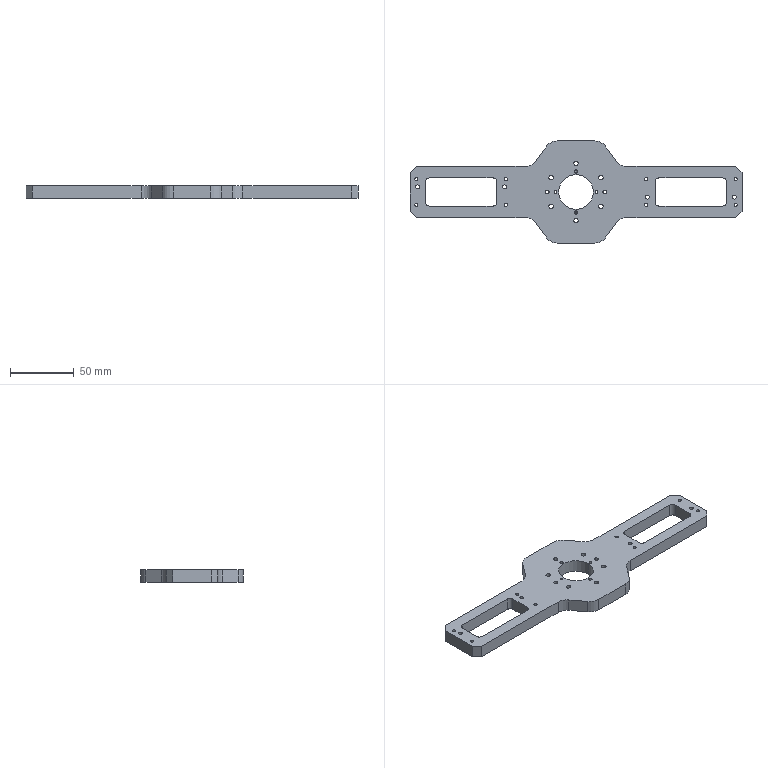CAM job | NX | 3-axis milling, drilling | part box 259.7 x 80 x 10 mm | stock box 265.7 x 86 x 11 mm
Tools:
number,name,description,diameter,corner_radius,flute_length,length,flutes
1,D63,Milling Tool-5 Parameters,63.0,0.0,50.0,75.0,2
7,D6A45,Milling Tool-5 Parameters,6.0,0.0,3.0,3.0,2
18,2.8ZT,Drilling Tool,2.8,0.0,35.0,50.0,2
19,3.0JD,Milling Tool-5 Parameters,3.0,0.0,30.0,30.0,4
8,2.5ZT,Drilling Tool,2.5,0.0,35.0,50.0,2
9,M3,Milling Tool-5 Parameters,2.5,0.0,30.0,30.0,4
13,3.5ZT,Drilling Tool,3.3,0.0,35.0,50.0,2
12,2.0ZT,Drilling Tool,2.0,0.0,35.0,50.0,2
10,D10,Milling Tool-5 Parameters,10.0,0.0,50.0,75.0,2
6,D6,Milling Tool-5 Parameters,6.0,0.0,50.0,75.0,2
11,D10JING,Milling Tool-5 Parameters,10.0,0.0,50.0,75.0,2
Operations:
program,operation,operation_type,tool,method,geometry_group,spindle_rpm,surface_speed,feed_per_tooth,feed_cut,feed_plunge,cut_length_mm,path_length_mm,cut_time_min,machine_time_min
1-263-83-10毛胚-AB胶,FLOOR_WALL,VolumeBased25DMillingOperation,D63,METHOD,A,6500.0,1286.0,0.0962,1250.0,100.0,1058.897,1112.897,0.8471,0.8525
1-263-83-10毛胚-AB胶,DRILLING_COPY_1,Operation,D6A45,METHOD,A,3000.0,56.0,0.0333,200.0,0.0,102.5,787.648,0.5125,0.581
1-263-83-10毛胚-AB胶,DRILLING_COPY_1_COPY_COPY_1,Operation,2.8ZT,METHOD,A,2000.0,15.0,0.0375,150.0,0.0,92.047,507.772,0.6136,0.6552
1-263-83-10毛胚-AB胶,DRILLING_COPY_1_COPY_COPY_1_COPY,Operation,3.0JD,METHOD,A,1000.0,9.0,0.0125,50.0,0.0,81.0,485.678,1.62,1.661
1-263-83-10毛胚-AB胶,DRILLING_COPY_1_COPY_1,Operation,2.5ZT,METHOD,A,2000.0,15.0,0.0375,150.0,0.0,146.511,743.703,0.9767,1.036
1-263-83-10毛胚-AB胶,DRILLING_COPY_1_COPY_COPY_2,Operation,M3,METHOD,A,200.0,1.0,0.125,100.0,0.0,131.0,712.681,1.31,1.368
1-263-83-10毛胚-AB胶,DRILLING_COPY_1_COPY_COPY_COPY_COPY_COPY,Operation,3.5ZT,METHOD,A,2000.0,20.0,0.0375,150.0,0.0,86.948,362.393,0.5797,0.6072
1-263-83-10毛胚-AB胶,DRILLING_COPY_1_COPY_COPY_COPY_COPY_COPY_COPY,Operation,2.0ZT,METHOD,A,2000.0,20.0,0.0375,150.0,0.0,28.202,151.544,0.188,0.2003
1-263-83-10毛胚-AB胶,ZLEVEL_PROFILE,ZLevelMilling,D10,METHOD,A,7000.0,219.0,0.2143,3000.0,1000.0,6641.161,6707.561,2.245,2.251
1-263-83-10毛胚-AB胶,ZLEVEL_PROFILE_COPY,ZLevelMilling,D10,METHOD,A,7000.0,219.0,0.2143,3000.0,1000.0,3137.374,3619.517,1.141,1.19
1-263-83-10毛胚-AB胶,ZLEVEL_PROFILE_COPY_1,ZLevelMilling,D6,METHOD,A,7000.0,87.0,0.1071,1500.0,1000.0,1553.638,2941.417,1.147,1.286
1-263-83-10毛胚-AB胶,ZLEVEL_PROFILE_COPY_COPY_1_COPY_COPY_COPY_1,ZLevelMilling,D6,METHOD,A,7000.0,219.0,0.0714,1000.0,100.0,336.191,820.779,0.3362,0.3846
1-263-83-10毛胚-AB胶,ZLEVEL_PROFILE_COPY_1_COPY_COPY_COPY_COPY_2_COPY_COPY_COPY,ZLevelMilling,D6A45,METHOD,A,7000.0,131.0,0.0714,1000.0,1000.0,1109.105,4312.035,1.109,1.429
1-263-83-10毛胚-AB胶,ZLEVEL_PROFILE_COPY_1_1,ZLevelMilling,D10JING,METHOD,A,7000.0,219.0,0.0714,1000.0,1000.0,2193.095,2259.845,2.193,2.2